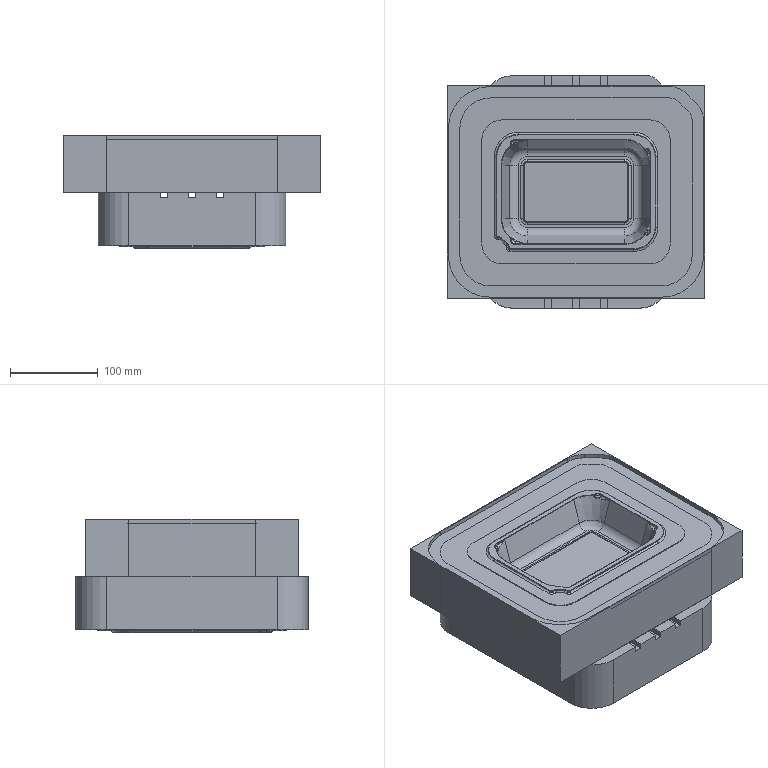NC program | NX | posted with a generic post | part box 293.342 x 265.342 x 129.5 mm
Lines 6051 to 7104 of 68427:
(B4 , TOOL : R2)
N12094 M6
N12096 G53
N12098 G17 G0 G90 X-64.361 Y-95.71 S9000 M3 M8
N12100 G43 Z215.5 H0
N12102 Z61.662
N12104 G94 G1 Z60.612 F30.
N12106 Y-90.515 F200.
N12108 X-64.521
N12110 X-64.769 Y-90.979
N12112 X-65.118 Y-91.279
N12114 X-65.572 Y-91.416
N12116 X-65.755 Y-91.425
N12118 X-66.113
N12120 Y-91.766
N12122 X-65.397
N12124 X-65.227 Y-91.809
N12126 X-65.118 Y-91.937
N12128 X-65.028 Y-92.079
N12130 X-65.011 Y-99.374
N12132 X-65.048 Y-99.559
N12134 X-65.11 Y-99.716
N12136 X-65.197 Y-99.844
N12138 X-65.292 Y-99.943
N12140 X-65.416 Y-100.014
N12142 X-65.571 Y-100.057
N12144 X-65.755 Y-100.071
N12146 X-66.113
N12148 Y-100.413
N12150 X-63.207
N12152 Y-100.071
N12154 X-63.605
N12156 X-63.774 Y-100.057
N12158 X-63.923 Y-100.014
N12160 X-64.053 Y-99.943
N12162 X-64.162 Y-99.844
N12164 X-64.249 Y-99.716
N12166 X-64.311 Y-99.559
N12168 X-64.349 Y-99.374
N12170 X-64.361 Y-99.161
N12172 Y-95.71
N12174 Z61.612
N12176 G0 Z215.5
N12178 X-54.606 Y-100.128
N12180 Z61.662
N12182 G1 Z60.612 F30.
N12184 X-54.853 Y-100.105 F200.
N12186 X-55.084 Y-100.037
N12188 X-55.299 Y-99.923
N12190 X-55.498 Y-99.764
N12192 X-55.681 Y-99.559
N12194 X-55.824 Y-99.318
N12196 X-55.936 Y-99.05
N12198 X-56.015 Y-98.754
N12200 X-56.063 Y-98.431
N12202 X-56.079 Y-98.08
N12204 X-55.993 Y-97.166
N12206 X-55.926 Y-96.879
N12208 X-55.84 Y-96.601
N12210 X-55.434 Y-95.864
N12212 X-55.267 Y-95.655
N12214 X-55.084 Y-95.464
N12216 X-54.721 Y-95.696
N12218 X-54.396 Y-95.937
N12220 X-54.109 Y-96.187
N12222 X-53.86 Y-96.447
N12224 X-53.65 Y-96.715
N12226 X-53.478 Y-96.991
N12228 X-53.344 Y-97.27
N12230 X-53.249 Y-97.555
N12232 X-53.192 Y-97.844
N12234 X-53.172 Y-98.137
N12236 X-53.187 Y-98.467
N12238 X-53.23 Y-98.774
N12240 X-53.301 Y-99.059
N12242 X-53.402 Y-99.32
N12244 X-53.531 Y-99.559
N12246 X-53.676 Y-99.764
N12248 X-53.856 Y-99.923
N12250 X-54.071 Y-100.037
N12252 X-54.321 Y-100.105
N12254 X-54.606 Y-100.128
N12256 Z61.612
N12258 G0 Z215.5
N12260 X-54.599 Y-100.526
N12262 Z61.662
N12264 G1 Z60.612 F30.
N12266 X-54.254 Y-100.497 F200.
N12268 X-53.931 Y-100.408
N12270 X-53.636 Y-100.26
N12272 X-53.37 Y-100.053
N12274 X-53.133 Y-99.787
N12276 X-52.932 Y-99.477
N12278 X-52.776 Y-99.141
N12280 X-52.664 Y-98.777
N12282 X-52.597 Y-98.385
N12284 X-52.575 Y-97.967
N12286 X-52.69 Y-97.052
N12288 X-53.035 Y-96.219
N12290 X-53.633 Y-95.468
N12292 X-53.889 Y-95.236
N12294 X-53.254 Y-94.649
N12296 X-52.859 Y-93.96
N12298 X-52.668 Y-93.175
N12300 X-52.655 Y-92.904
N12302 X-52.675 Y-92.529
N12304 X-52.738 Y-92.176
N12306 X-52.841 Y-91.846
N12308 X-52.986 Y-91.539
N12310 X-53.172 Y-91.254
N12312 X-53.392 Y-91.009
N12314 X-53.637 Y-90.818
N12316 X-53.908 Y-90.681
N12318 X-54.204 Y-90.599
N12320 X-54.526 Y-90.572
N12322 X-54.877 Y-90.599
N12324 X-55.195 Y-90.681
N12326 X-55.482 Y-90.818
N12328 X-55.737 Y-91.009
N12330 X-55.96 Y-91.254
N12332 X-56.146 Y-91.539
N12334 X-56.291 Y-91.846
N12336 X-56.394 Y-92.176
N12338 X-56.457 Y-92.529
N12340 X-56.477 Y-92.904
N12342 X-56.377 Y-93.75
N12344 X-56.299 Y-94.014
N12346 X-56.199 Y-94.269
N12348 X-55.73 Y-94.89
N12350 X-55.536 Y-95.07
N12352 X-55.323 Y-95.236
N12354 X-55.987 Y-95.912
N12356 X-56.164 Y-96.165
N12358 X-56.318 Y-96.431
N12360 X-56.433 Y-96.715
N12362 X-56.522 Y-97.022
N12364 X-56.637 Y-98.08
N12366 X-56.613 Y-98.458
N12368 X-56.541 Y-98.818
N12370 X-56.422 Y-99.159
N12372 X-56.254 Y-99.482
N12374 X-56.039 Y-99.787
N12376 X-55.791 Y-100.053
N12378 X-55.523 Y-100.26
N12380 X-55.237 Y-100.408
N12382 X-54.931 Y-100.497
N12384 X-54.606 Y-100.526
N12386 X-54.599
N12388 Z61.612
N12390 G0 Z63.662
N12392 X-53.212 Y-92.961
N12394 Z61.662
N12396 G1 Z60.612 F30.
N12398 X-53.298 Y-93.719 F200.
N12400 X-53.556 Y-94.353
N12402 X-53.986 Y-94.865
N12404 X-54.168 Y-95.009
N12406 X-55.042 Y-94.422
N12408 X-55.276 Y-94.208
N12410 X-55.482 Y-93.985
N12412 X-55.64 Y-93.735
N12414 X-55.762 Y-93.484
N12416 X-55.85 Y-93.234
N12418 X-55.902 Y-92.984
N12420 X-55.869 Y-92.242
N12422 X-55.601 Y-91.539
N12424 X-55.456 Y-91.334
N12426 X-55.276 Y-91.175
N12428 X-55.061 Y-91.061
N12430 X-54.811 Y-90.993
N12432 X-54.526 Y-90.97
N12434 X-54.27 Y-90.995
N12436 X-54.042 Y-91.07
N12438 X-53.843 Y-91.195
N12440 X-53.673 Y-91.37
N12442 X-53.531 Y-91.596
N12444 X-53.416 Y-91.832
N12446 X-53.327 Y-92.087
N12448 X-53.212 Y-92.961
N12450 Z61.612
N12452 G0 Z215.5
N12454 X-44.412 Y-100.128
N12456 Z61.662
N12458 G1 Z60.612 F30.
N12460 X-44.659 Y-100.105 F200.
N12462 X-44.89 Y-100.037
N12464 X-45.105 Y-99.923
N12466 X-45.304 Y-99.764
N12468 X-45.488 Y-99.559
N12470 X-45.631 Y-99.318
N12472 X-45.742 Y-99.05
N12474 X-45.822 Y-98.754
N12476 X-45.87 Y-98.431
N12478 X-45.886 Y-98.08
N12480 X-45.8 Y-97.166
N12482 X-45.733 Y-96.879
N12484 X-45.647 Y-96.601
N12486 X-45.241 Y-95.864
N12488 X-45.073 Y-95.655
N12490 X-44.89 Y-95.464
N12492 X-44.527 Y-95.696
N12494 X-44.202 Y-95.937
N12496 X-43.916 Y-96.187
N12498 X-43.667 Y-96.447
N12500 X-43.457 Y-96.715
N12502 X-43.285 Y-96.991
N12504 X-43.151 Y-97.27
N12506 X-43.055 Y-97.555
N12508 X-42.998 Y-97.844
N12510 X-42.979 Y-98.137
N12512 X-42.993 Y-98.467
N12514 X-43.036 Y-98.774
N12516 X-43.108 Y-99.059
N12518 X-43.208 Y-99.32
N12520 X-43.337 Y-99.559
N12522 X-43.482 Y-99.764
N12524 X-43.662 Y-99.923
N12526 X-43.877 Y-100.037
N12528 X-44.127 Y-100.105
N12530 X-44.412 Y-100.128
N12532 Z61.612
N12534 G0 Z215.5
N12536 X-44.406 Y-100.526
N12538 Z61.662
N12540 G1 Z60.612 F30.
N12542 X-44.06 Y-100.497 F200.
N12544 X-43.737 Y-100.408
N12546 X-43.442 Y-100.26
N12548 X-43.177 Y-100.053
N12550 X-42.939 Y-99.787
N12552 X-42.739 Y-99.477
N12554 X-42.582 Y-99.141
N12556 X-42.471 Y-98.777
N12558 X-42.404 Y-98.385
N12560 X-42.382 Y-97.967
N12562 X-42.496 Y-97.052
N12564 X-42.842 Y-96.219
N12566 X-43.439 Y-95.468
N12568 X-43.696 Y-95.236
N12570 X-43.06 Y-94.649
N12572 X-42.665 Y-93.96
N12574 X-42.474 Y-93.175
N12576 X-42.461 Y-92.904
N12578 X-42.482 Y-92.529
N12580 X-42.544 Y-92.176
N12582 X-42.648 Y-91.846
N12584 X-42.793 Y-91.539
N12586 X-42.979 Y-91.254
N12588 X-43.199 Y-91.009
N12590 X-43.444 Y-90.818
N12592 X-43.715 Y-90.681
N12594 X-44.011 Y-90.599
N12596 X-44.333 Y-90.572
N12598 X-44.683 Y-90.599
N12600 X-45.002 Y-90.681
N12602 X-45.288 Y-90.818
N12604 X-45.543 Y-91.009
N12606 X-45.766 Y-91.254
N12608 X-45.953 Y-91.539
N12610 X-46.098 Y-91.846
N12612 X-46.201 Y-92.176
N12614 X-46.263 Y-92.529
N12616 X-46.284 Y-92.904
N12618 X-46.184 Y-93.75
N12620 X-46.106 Y-94.014
N12622 X-46.005 Y-94.269
N12624 X-45.537 Y-94.89
N12626 X-45.343 Y-95.07
N12628 X-45.129 Y-95.236
N12630 X-45.793 Y-95.912
N12632 X-45.97 Y-96.165
N12634 X-46.125 Y-96.431
N12636 X-46.239 Y-96.715
N12638 X-46.329 Y-97.022
N12640 X-46.443 Y-98.08
N12642 X-46.419 Y-98.458
N12644 X-46.348 Y-98.818
N12646 X-46.228 Y-99.159
N12648 X-46.061 Y-99.482
N12650 X-45.846 Y-99.787
N12652 X-45.597 Y-100.053
N12654 X-45.33 Y-100.26
N12656 X-45.043 Y-100.408
N12658 X-44.737 Y-100.497
N12660 X-44.412 Y-100.526
N12662 X-44.406
N12664 Z61.612
N12666 G0 Z63.662
N12668 X-43.019 Y-92.961
N12670 Z61.662
N12672 G1 Z60.612 F30.
N12674 X-43.105 Y-93.719 F200.
N12676 X-43.363 Y-94.353
N12678 X-43.793 Y-94.865
N12680 X-43.974 Y-95.009
N12682 X-44.849 Y-94.422
N12684 X-45.083 Y-94.208
N12686 X-45.288 Y-93.985
N12688 X-45.446 Y-93.735
N12690 X-45.569 Y-93.484
N12692 X-45.656 Y-93.234
N12694 X-45.709 Y-92.984
N12696 X-45.675 Y-92.242
N12698 X-45.408 Y-91.539
N12700 X-45.263 Y-91.334
N12702 X-45.083 Y-91.175
N12704 X-44.868 Y-91.061
N12706 X-44.618 Y-90.993
N12708 X-44.333 Y-90.97
N12710 X-44.076 Y-90.995
N12712 X-43.849 Y-91.07
N12714 X-43.65 Y-91.195
N12716 X-43.479 Y-91.37
N12718 X-43.337 Y-91.596
N12720 X-43.223 Y-91.832
N12722 X-43.134 Y-92.087
N12724 X-43.019 Y-92.961
N12726 Z61.612
N12728 G0 Z215.5
N12730 X-35.177 Y-98.06
N12732 Z61.662
N12734 G1 Z60.612 F30.
N12736 X-35.653 Y-99.502 F200.
N12738 X-35.714 Y-99.648
N12740 X-36.002 Y-99.995
N12742 X-36.121 Y-100.052
N12744 X-36.25 Y-100.071
N12746 X-36.409
N12748 Y-100.413
N12750 X-34.896
N12752 Y-100.071
N12754 X-35.254 Y-100.014
N12756 X-35.314 Y-99.872
N12758 X-35.334 Y-99.673
N12760 X-35.135 Y-98.934
N12762 X-34.219 Y-96.203
N12764 X-33.144 Y-99.559
N12766 X-33.104 Y-99.773
N12768 X-33.144 Y-99.958
N12770 X-33.224 Y-100.043
N12772 X-33.383 Y-100.071
N12774 X-33.542
N12776 Y-100.413
N12778 X-31.83
N12780 Y-100.071
N12782 X-31.949
N12784 X-32.109 Y-100.043
N12786 X-32.268 Y-99.958
N12788 X-32.507 Y-99.446
N12790 X-33.901 Y-95.179
N12792 X-32.666 Y-91.482
N12794 X-32.427 Y-91.141
N12796 X-32.318 Y-91.055
N12798 X-32.228 Y-91.027
N12800 X-31.989
N12802 Y-90.686
N12804 X-33.542
N12806 Y-91.027
N12808 X-33.303
N12810 X-33.166 Y-91.052
N12812 X-33.073 Y-91.128
N12814 X-33.025 Y-91.254
N12816 X-33.016 Y-91.393
N12818 X-33.042 Y-91.583
N12820 X-33.104 Y-91.823
N12822 X-34.06 Y-94.724
N12824 X-35.015 Y-91.71
N12826 X-35.055 Y-91.501
N12828 X-35.069 Y-91.33
N12830 X-35.055 Y-91.198
N12832 X-34.966 Y-91.07
N12834 X-34.777 Y-91.027
N12836 X-34.657
N12838 Y-90.686
N12840 X-36.29
N12842 Y-91.027
N12844 X-36.13
N12846 X-35.991 Y-91.055
N12848 X-35.891 Y-91.141
N12850 X-35.792 Y-91.269
N12852 X-35.732 Y-91.425
N12854 X-34.378 Y-95.634
N12856 X-35.177 Y-98.06
N12858 Z61.612
N12860 G0 Z215.5
N12862 X-23.588 Y-95.71
N12864 Z61.662
N12866 G1 Z60.612 F30.
N12868 Y-90.515 F200.
N12870 X-23.747
N12872 X-23.995 Y-90.979
N12874 X-24.344 Y-91.279
N12876 X-24.798 Y-91.416
N12878 X-24.981 Y-91.425
N12880 X-25.34
N12882 Y-91.766
N12884 X-24.623
N12886 X-24.454 Y-91.809
N12888 X-24.344 Y-91.937
N12890 X-24.255 Y-92.079
N12892 X-24.237 Y-99.374
N12894 X-24.275 Y-99.559
N12896 X-24.337 Y-99.716
N12898 X-24.424 Y-99.844
N12900 X-24.518 Y-99.943
N12902 X-24.643 Y-100.014
N12904 X-24.797 Y-100.057
N12906 X-24.981 Y-100.071
N12908 X-25.34
N12910 Y-100.413
N12912 X-22.433
N12914 Y-100.071
N12916 X-22.831
N12918 X-23. Y-100.057
N12920 X-23.15 Y-100.014
N12922 X-23.279 Y-99.943
N12924 X-23.389 Y-99.844
N12926 X-23.476 Y-99.716
N12928 X-23.538 Y-99.559
N12930 X-23.575 Y-99.374
N12932 X-23.588 Y-99.161
N12934 Y-95.71
N12936 Z61.612
N12938 G0 Z215.5
N12940 X-15.642 Y-98.279
N12942 Z61.662
N12944 G1 Z60.612 F30.
N12946 X-15.686 Y-98.434 F200.
N12948 X-15.704 Y-98.649
N12950 X-15.683 Y-98.938
N12952 X-15.621 Y-99.213
N12954 X-15.517 Y-99.475
N12956 X-15.372 Y-99.723
N12958 X-15.186 Y-99.958
N12960 X-14.971 Y-100.162
N12962 X-14.74 Y-100.322
N12964 X-14.493 Y-100.435
N12966 X-14.23 Y-100.504
N12968 X-13.952 Y-100.526
N12970 X-13.571 Y-100.494
N12972 X-13.225 Y-100.399
N12974 X-12.915 Y-100.24
N12976 X-12.639 Y-100.017
N12978 X-12.399 Y-99.73
N12980 X-12.198 Y-99.38
N12982 X-12.042 Y-99.011
N12984 X-11.931 Y-98.624
N12986 X-11.864 Y-98.219
N12988 X-11.841 Y-97.796
N12990 X-11.854 Y-97.5
N12992 X-12.045 Y-96.613
N12994 X-12.16 Y-96.317
N12996 X-12.31 Y-96.033
N12998 X-12.504 Y-95.771
N13000 X-12.743 Y-95.532
N13002 X-13.026 Y-95.316
N13004 X-13.354 Y-95.122
N13006 X-13.114 Y-94.997
N13008 X-12.902 Y-94.849
N13010 X-12.719 Y-94.679
N13012 X-12.564 Y-94.485
N13014 X-12.235 Y-93.732
N13016 X-12.12 Y-92.79
N13018 X-12.139 Y-92.476
N13020 X-12.197 Y-92.171
N13022 X-12.292 Y-91.876
N13024 X-12.426 Y-91.589
N13026 X-12.598 Y-91.311
N13028 X-12.802 Y-91.045
N13030 X-13.031 Y-90.838
N13032 X-13.286 Y-90.69
N13034 X-13.566 Y-90.601
N13036 X-13.872 Y-90.572
N13038 X-14.136 Y-90.595
N13040 X-14.388 Y-90.663
N13042 X-14.627 Y-90.777
N13044 X-14.853 Y-90.936
N13046 X-15.067 Y-91.141
N13048 X-15.253 Y-91.359
N13050 X-15.398 Y-91.605
N13052 X-15.501 Y-91.878
N13054 X-15.564 Y-92.178
N13056 X-15.584 Y-92.506
N13058 X-15.571 Y-92.778
N13060 X-15.531 Y-92.986
N13062 X-15.465 Y-93.132
N13064 X-15.359 Y-93.226
N13066 X-15.252 Y-93.283
N13068 X-15.146 Y-93.302
N13070 X-14.977 Y-93.26
N13072 X-14.868 Y-93.132
N13074 X-14.808 Y-92.932
N13076 X-14.788 Y-92.677
N13078 X-14.938 Y-92.089
N13080 X-14.947 Y-91.823
N13082 X-14.927 Y-91.614
N13084 X-14.868 Y-91.439
N13086 X-14.768 Y-91.301
N13088 X-14.32 Y-91.027
N13090 X-14.173 Y-90.984
N13092 X-14.031 Y-90.97
N13094 X-13.791 Y-90.995
N13096 X-13.579 Y-91.07
N13098 X-13.396 Y-91.195
N13100 X-13.241 Y-91.37
N13102 X-12.912 Y-92.087
N13104 X-12.797 Y-92.961
N13106 X-12.813 Y-93.332
N13108 X-12.861 Y-93.671
N13110 X-12.94 Y-93.978
N13112 X-13.052 Y-94.253
N13114 X-13.195 Y-94.497
N13116 X-13.356 Y-94.681
N13118 X-13.552 Y-94.824
N13120 X-13.783 Y-94.927
N13122 X-14.049 Y-94.988
N13124 X-14.35 Y-95.009
N13126 Y-95.407
N13128 X-13.963 Y-95.432
N13130 X-13.63 Y-95.507
N13132 X-13.351 Y-95.632
N13134 X-13.127 Y-95.807
N13136 X-12.956 Y-96.033
N13138 X-12.813 Y-96.299
N13140 X-12.701 Y-96.597
N13142 X-12.622 Y-96.927
N13144 X-12.574 Y-97.289
N13146 X-12.558 Y-97.682
N13148 X-12.572 Y-98.158
N13150 X-12.615 Y-98.583
N13152 X-12.687 Y-98.959
N13154 X-12.787 Y-99.284
N13156 X-12.916 Y-99.559
N13158 X-13.074 Y-99.764
N13160 X-13.26 Y-99.923
N13162 X-13.475 Y-100.037
N13164 X-13.719 Y-100.105
N13166 X-14.272 Y-100.092
N13168 X-14.668 Y-99.901
N13170 X-14.79 Y-99.78
N13172 X-14.877 Y-99.645
N13174 X-14.93 Y-99.495
N13176 X-14.947 Y-99.332
N13178 X-14.797 Y-98.662
N13180 X-14.788 Y-98.479
N13182 X-14.818 Y-98.294
N13184 X-14.907 Y-98.08
N13186 X-14.978 Y-97.922
N13188 X-15.084 Y-97.828
N13190 X-15.226 Y-97.796
N13192 X-15.332 Y-97.828
N13194 X-15.438 Y-97.922
N13196 X-15.642 Y-98.279
N13198 Z61.612
N13200 G0 Z215.5
N13202 X-3.515 Y-100.347
N13204 Z61.662
N13206 G1 Z60.612 F30.
N13208 X-3.453 Y-100.21 F200.
N13210 X-3.413 Y-100.002
N13212 X-3.421 Y-97.516
N13214 X-3.363 Y-96.915
N13216 X-3.268 Y-96.278
N13218 X-3.134 Y-95.605
N13220 X-2.962 Y-94.895
N13222 X-2.226 Y-92.622
N13224 X-1.93 Y-91.855
N13226 X-1.608 Y-91.084
N13228 Y-90.686
N13230 X-5.192
N13232 X-5.47 Y-93.075
N13234 X-5.232 Y-93.132
N13236 X-5.045 Y-92.319
N13238 X-4.964 Y-92.112
N13240 X-4.873 Y-91.937
N13242 X-4.755 Y-91.794
N13244 X-4.625 Y-91.682
N13246 X-4.481 Y-91.603
N13248 X-4.325 Y-91.555
N13250 X-4.156 Y-91.539
N13252 X-2.166
N13254 X-3.532 Y-95.314
N13256 X-3.809 Y-96.217
N13258 X-3.997 Y-96.943
N13260 X-4.265 Y-98.67
N13262 X-4.308 Y-99.854
N13264 X-4.196 Y-100.356
N13266 X-4.086 Y-100.451
N13268 X-3.966 Y-100.507
N13270 X-3.838 Y-100.526
N13272 X-3.696 Y-100.507
N13274 X-3.515 Y-100.347
N13276 Z61.612
N13278 G0 Z215.5
N13280 X9.979 Y-100.635
N13282 Z61.662
N13284 G1 Z60.612 F30.
N13286 Y-101.323 F200.
N13288 X10.011 Y-101.769
N13290 X10.106 Y-102.105
N13292 X10.266 Y-102.333
N13294 X10.489 Y-102.451
N13296 X10.775 Y-102.46
N13298 X12.607
N13300 X13.005 Y-102.351
N13302 X13.308 Y-101.932
N13304 X13.515 Y-101.204
N13306 X13.626 Y-100.167
N13308 X13.642 Y-98.82
N13310 X13.523 Y-98.649
N13312 X13.403 Y-98.592
N13314 X13.284 Y-98.649
N13316 X13.164 Y-98.82
N13318 Y-99.921
N13320 X13.101 Y-100.768
N13322 X12.973 Y-101.359
N13324 X12.782 Y-101.696
N13326 X12.527 Y-101.778
N13328 X10.935
N13330 X10.763 Y-101.787
N13332 X10.629 Y-101.723
N13334 X10.533 Y-101.587
N13336 X10.476 Y-101.377
N13338 X10.457 Y-101.095
N13340 Y-96.089
N13342 X13.801
N13344 X13.921 Y-95.919
N13346 X13.961 Y-95.748
N13348 X13.921 Y-95.578
N13350 X13.801 Y-95.407
N13352 X10.457
N13354 Y-91.084
N13356 X11.967 Y-90.729
N13358 X12.419 Y-90.574
N13360 X12.846 Y-90.401
N13362 X12.925 Y-90.145
N13364 Y-89.946
N13366 X12.846 Y-89.804
N13368 X12.687 Y-89.719
N13370 X11.877 Y-90.019
N13372 X10.979 Y-90.283
N13374 X9.992 Y-90.51
N13376 X8.915 Y-90.702
N13378 X7.749 Y-90.856
N13380 X7.664 Y-91.07
N13382 X7.65 Y-91.254
N13384 X7.704 Y-91.411
N13386 X7.829 Y-91.539
N13388 X9.979 Y-91.198
N13390 Y-95.407
N13392 X7.749
N13394 X7.63 Y-95.62
N13396 X7.59 Y-95.805
N13398 X7.63 Y-95.961
N13400 X7.749 Y-96.089
N13402 X9.979
N13404 Y-100.635
N13406 Z61.612
N13408 G0 Z215.5
N13410 X6.475 Y-100.994
N13412 Z61.662
N13414 G1 Z60.612 F30.
N13416 Y-97.682 F200.
N13418 X7.669 Y-96.886
N13420 X7.736 Y-96.677
N13422 X7.746 Y-96.504
N13424 X7.698 Y-96.367
N13426 X7.593 Y-96.267
N13428 X7.431 Y-96.203
N13430 X6.475 Y-96.886
N13432 Y-92.904
N13434 X7.749
N13436 X7.898 Y-92.733
N13438 X7.948 Y-92.563
N13440 X7.898 Y-92.392
N13442 X7.749 Y-92.221
N13444 X6.475
N13446 Y-89.491
N13448 X6.355 Y-89.32
N13450 X6.236 Y-89.264
N13452 X6.117 Y-89.32
N13454 X5.997 Y-89.491
N13456 Y-92.221
N13458 X4.404
N13460 X4.285 Y-92.392
N13462 X4.245 Y-92.563
N13464 X4.285 Y-92.733
N13466 X4.404 Y-92.904
N13468 X5.997
N13470 Y-97.113
N13472 X4.825 Y-97.696
N13474 X4.564 Y-97.796
N13476 X4.484 Y-98.052
N13478 Y-98.251
N13480 X4.564 Y-98.393
N13482 X4.723 Y-98.479
N13484 X5.997 Y-97.91
N13486 Y-101.323
N13488 X5.972 Y-101.573
N13490 X5.831 Y-101.687
N13492 X5.577 Y-101.664
N13494 X5.207 Y-101.505
N13496 X4.723 Y-101.209
N13498 X4.56 Y-101.236
N13500 X4.455 Y-101.318
N13502 X4.408 Y-101.455
N13504 X4.417 Y-101.646
N13506 X4.484 Y-101.892
N13508 X4.771 Y-102.096
N13510 X5.057 Y-102.256
N13512 X5.344 Y-102.369
N13514 X5.631 Y-102.438
N13516 X5.917 Y-102.46
N13518 X6.144 Y-102.383
N13520 X6.312 Y-102.242
N13522 X6.424 Y-102.037
N13524 X6.478 Y-101.769
N13526 X6.475 Y-101.436
N13528 Y-100.994
N13530 Z61.612
N13532 G0 Z215.5
N13534 X16.652 Y-91.026
N13536 Z61.662
N13538 G1 Z60.612 F30.
N13540 X16.621 Y-91.129 F200.
N13542 X16.589 Y-91.539
N13544 Y-93.587
N13546 X15.235
N13548 X15.086 Y-93.757
N13550 X15.036 Y-93.928
N13552 X15.086 Y-94.099
N13554 X15.235 Y-94.269
N13556 X16.589
N13558 Y-94.975
N13560 X16.525 Y-95.634
N13562 X16.398 Y-96.249
N13564 X16.206 Y-96.818
N13566 X15.952 Y-97.341
N13568 X15.976 Y-97.618
N13570 X16.051 Y-97.768
N13572 X16.176 Y-97.789
N13574 X16.35 Y-97.682
N13576 X16.633 Y-97.145
N13578 X16.847 Y-96.535
N13580 X16.99 Y-95.853
N13582 X17.063 Y-95.097
N13584 X17.066 Y-94.269
N13586 X21.845
N13588 Y-96.431
N13590 X21.854 Y-96.736
N13592 X21.755 Y-96.922
N13594 X21.548 Y-96.991
N13596 X21.233 Y-96.94
N13598 X20.809 Y-96.772
N13600 X20.655 Y-96.9
N13602 X20.59 Y-97.056
N13604 X20.615 Y-97.241
N13606 X20.73 Y-97.455
N13608 X21.329 Y-97.641
N13610 X21.787 Y-97.655
N13612 X22.106 Y-97.496
N13614 X22.284 Y-97.163
N13616 X22.322 Y-96.658
N13618 Y-94.269
N13620 X23.597
N13622 X23.746 Y-94.099
N13624 X23.796 Y-93.928
N13626 X23.746 Y-93.757
N13628 X23.597 Y-93.587
N13630 X22.322
N13632 Y-91.539
N13634 X22.316 Y-91.129
N13636 X22.233 Y-90.811
N13638 X22.074 Y-90.583
N13640 X21.838 Y-90.447
N13642 X21.526 Y-90.401
N13644 X19.456
N13646 X19.774 Y-89.377
N13648 X19.704 Y-89.154
N13650 X19.621 Y-89.031
N13652 X19.526 Y-89.009
N13654 X19.417 Y-89.086
N13656 X19.296 Y-89.264
N13658 X18.898 Y-90.401
N13660 X17.385
N13662 X17.098 Y-90.447
N13664 X16.875 Y-90.583
N13666 X16.716 Y-90.811
N13668 X16.652 Y-91.026
N13670 Z61.612
N13672 G0 Z63.662
N13674 X21.367 Y-91.084
N13676 Z61.662
N13678 G1 Z60.612 F30.
N13680 X21.564 Y-91.111 F200.
N13682 X21.711 Y-91.193
N13684 X21.806 Y-91.33
N13686 X21.851 Y-91.521
N13688 X21.845 Y-91.766
N13690 Y-93.587
N13692 X17.066
N13694 Y-91.766
N13696 X17.086 Y-91.521
N13698 X17.143 Y-91.33
N13700 X17.239 Y-91.193
N13702 X17.372 Y-91.111
N13704 X17.544 Y-91.084
N13706 X21.367
N13708 Z61.612
N13710 G0 Z215.5
N13712 X19.753 Y-92.305
N13714 Z61.662
N13716 G1 Z60.612 F30.
N13718 X19.057 Y-91.311 F200.
N13720 X18.892 Y-91.298
N13722 X18.777 Y-91.348
N13724 X18.713 Y-91.461
N13726 X18.701 Y-91.639
N13728 X18.739 Y-91.88
N13730 X19.35 Y-92.74
N13732 X19.529 Y-93.045
N13734 X19.694 Y-93.359
N13736 X19.863 Y-93.414
N13738 X19.988 Y-93.396
N13740 X20.067 Y-93.305
N13742 X20.102 Y-93.141
N13744 X20.093 Y-92.904
N13746 X19.898 Y-92.549
N13748 X19.753 Y-92.305
N13750 Z61.612
N13752 G0 Z215.5
N13754 X19.312 Y-98.137
N13756 Z61.662
N13758 G1 Z60.612 F30.
N13760 X16.429 F200.
N13762 X16.143 Y-98.183
N13764 X15.92 Y-98.319
N13766 X15.76 Y-98.547
N13768 X15.665 Y-98.865
N13770 X15.633 Y-99.275
N13772 Y-101.778
N13774 X14.837
N13776 X14.687 Y-101.948
N13778 X14.638 Y-102.119
N13780 X14.687 Y-102.29
N13782 X14.837 Y-102.46
N13784 X23.915
N13786 X24.065 Y-102.29
N13788 X24.114 Y-102.119
N13790 X24.065 Y-101.948
N13792 X23.915 Y-101.778
N13794 X22.96
N13796 Y-99.275
N13798 X22.953 Y-98.865
N13800 X22.87 Y-98.547
N13802 X22.711 Y-98.319
N13804 X22.475 Y-98.183
N13806 X22.163 Y-98.137
N13808 X19.312
N13810 Z61.612
N13812 G0 Z63.662
N13814 X18.022 Y-98.82
N13816 Z61.662
N13818 G1 Z60.612 F30.
N13820 Y-101.778 F200.
N13822 X16.111
N13824 Y-99.502
N13826 X16.13 Y-99.257
N13828 X16.187 Y-99.066
N13830 X16.283 Y-98.929
N13832 X16.417 Y-98.847
N13834 X16.589 Y-98.82
N13836 X18.022
N13838 Z61.612
N13840 G0 Z63.662
N13842 X20.252
N13844 Z61.662
N13846 G1 Z60.612 F30.
N13848 Y-101.778 F200.
N13850 X18.5
N13852 Y-98.82
N13854 X20.252
N13856 Z61.612
N13858 G0 Z63.662
N13860 X22.004
N13862 Z61.662
N13864 G1 Z60.612 F30.
N13866 X22.201 Y-98.847 F200.
N13868 X22.348 Y-98.929
N13870 X22.444 Y-99.066
N13872 X22.488 Y-99.257
N13874 X22.482 Y-99.502
N13876 Y-101.778
N13878 X20.73
N13880 Y-98.82
N13882 X22.004
N13884 Z61.612
N13886 G0 Z215.5
N13888 X19.596 Y-95.219
N13890 Z61.662
N13892 G1 Z60.612 F30.
N13894 X18.978 Y-94.497 F200.
N13896 X18.812 Y-94.483
N13898 X18.697 Y-94.533
N13900 X18.634 Y-94.647
N13902 X18.621 Y-94.824
N13904 X18.659 Y-95.066
N13906 X19.774 Y-96.431
N13908 X19.948 Y-96.488
N13910 X20.073 Y-96.431
N13912 X20.147 Y-96.26
N13914 X20.172 Y-95.976
N13916 X19.596 Y-95.219
N13918 Z61.612
N13920 G0 Z215.5
N13922 X30.844 Y-100.754
N13924 Z61.662
N13926 G1 Z60.612 F30.
N13928 Y-102.46 F200.
N13930 X30.963 Y-102.631
N13932 X31.082 Y-102.688
N13934 X31.202 Y-102.631
N13936 X31.321 Y-102.46
N13938 Y-99.047
N13940 X34.188
N13942 X34.308 Y-98.877
N13944 X34.347 Y-98.706
N13946 X34.308 Y-98.535
N13948 X34.188 Y-98.365
N13950 X31.321
N13952 Y-95.748
N13954 X33.71
N13956 X33.83 Y-95.578
N13958 X33.87 Y-95.407
N13960 X33.83 Y-95.236
N13962 X33.71 Y-95.066
N13964 X31.321
N13966 Y-92.449
N13968 X33.71
N13970 X33.83 Y-92.278
N13972 X33.87 Y-92.108
N13974 X33.83 Y-91.937
N13976 X33.71 Y-91.766
N13978 X32.197
N13980 X33.073 Y-89.377
N13982 X32.984 Y-89.15
N13984 X32.874 Y-89.036
N13986 X32.745
N13988 X32.596 Y-89.15
N13990 X32.06 Y-90.747
N13992 X31.856 Y-91.261
N13994 X31.64 Y-91.766
N13996 X28.454
N13998 X28.335 Y-91.937
N14000 X28.295 Y-92.108
N14002 X28.335 Y-92.278
N14004 X28.454 Y-92.449
N14006 X30.844
N14008 Y-95.066
N14010 X28.614
N14012 X28.494 Y-95.236
N14014 X28.454 Y-95.407
N14016 X28.494 Y-95.578
N14018 X28.614 Y-95.748
N14020 X30.844
N14022 Y-98.365
N14024 X28.295
N14026 X28.176 Y-98.535
N14028 X28.136 Y-98.706
N14030 X28.176 Y-98.877
N14032 X28.295 Y-99.047
N14034 X30.844
N14036 Y-100.754
N14038 Z61.612
N14040 G0 Z215.5
N14042 X26.862 Y-98.365
N14044 Z61.662
N14046 G1 Z60.612 F30.
N14048 Y-94.269 F200.
N14050 X27.575 Y-96.636
N14052 X27.658 Y-97.
N14054 X27.832 Y-97.056
N14056 X27.957 Y-97.
N14058 X28.031 Y-96.829
N14060 X28.056 Y-96.545
N14062 X27.215 Y-93.705
N14064 X26.941 Y-92.904
N14066 X27.977
N14068 X28.096 Y-92.733
N14070 X28.136 Y-92.563
N14072 X28.096 Y-92.392
N14074 X27.977 Y-92.221
N14076 X26.862
N14078 Y-89.491
N14080 X26.742 Y-89.32
N14082 X26.623 Y-89.264
N14084 X26.503 Y-89.32
N14086 X26.384 Y-89.491
N14088 Y-92.221
N14090 X25.03
N14092 X24.911 Y-92.392
N14094 X24.871 Y-92.563
N14096 X24.911 Y-92.733
N14098 X25.03 Y-92.904
N14100 X26.225
N14102 X26.037 Y-94.101
N14104 X25.791 Y-95.234
N14106 X25.489 Y-96.303
N14108 X25.129 Y-97.309
N14110 X24.712 Y-98.251
N14112 X24.707 Y-98.493
N14114 X24.771 Y-98.649
N14116 X24.906 Y-98.72
N14118 X25.11 Y-98.706
N14120 X25.466 Y-97.932
N14122 X25.772 Y-97.159
N14124 X26.027 Y-96.385
N14126 X26.231 Y-95.612
N14128 X26.384 Y-94.838
N14130 Y-102.46
N14132 X26.503 Y-102.631
N14134 X26.623 Y-102.688
N14136 X26.742 Y-102.631
N14138 X26.862 Y-102.46
N14140 Y-98.365
N14142 Z61.612
N14144 G0 Z215.5
N14146 X29.915 Y-90.298
N14148 Z61.662
N14150 G1 Z60.612 F30.
N14152 X29.41 Y-89.15 F200.
N14154 X29.206 Y-89.136
N14156 X29.072 Y-89.207
N14158 X29.007 Y-89.363
N14160 X29.012 Y-89.605
N14162 X29.649 Y-91.097
N14164 X29.808 Y-91.539
N14166 X29.982 Y-91.553
N14168 X30.107 Y-91.482
N14170 X30.182 Y-91.326
N14172 X30.206 Y-91.084
N14174 X30.047 Y-90.642
N14176 X29.915 Y-90.298
N14178 Z61.612
N14180 G0 Z215.5
N14182 X37.135 Y-89.491
N14184 Z61.662
N14186 G1 Z60.612 F30.
N14188 X36.848 Y-89.573 F200.
N14190 X36.625 Y-89.728
N14192 X36.466 Y-89.955
N14194 X36.37 Y-90.256